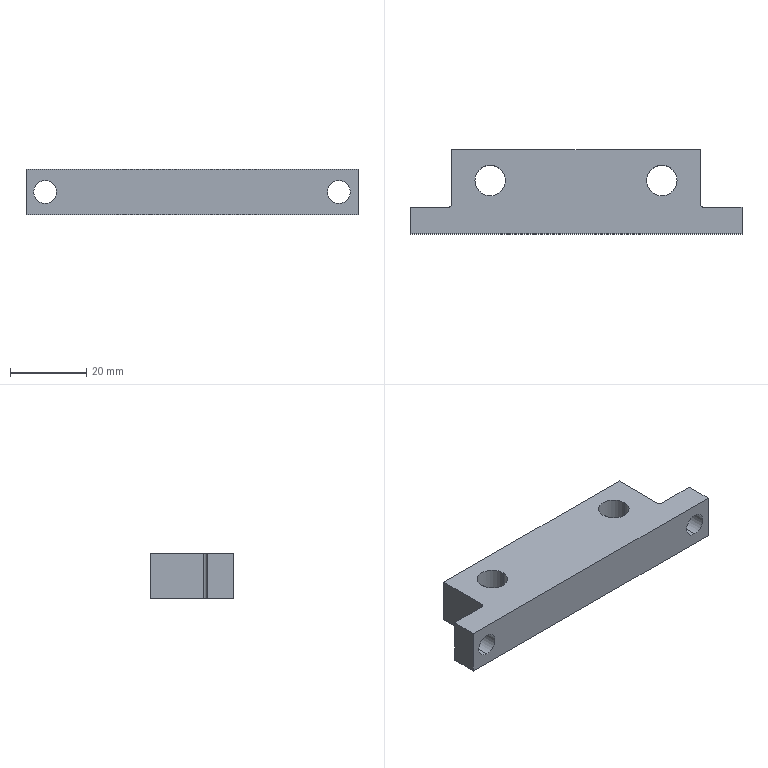Part | SolidWorks | features 3DProfileFeature 1, Extrusion 1, Fillet 1, HoleWzd 1, ICE 1, MirrorPattern 1 | 1 solid | 24 faces | box 87 x 22 x 12 mm | volume 17341 mm3 | cylinder 14 | plane 10 | commonest cylinder face diameters 3.3 x4 6 x4 8 x4 2 x2
STEP:
#1=CARTESIAN_POINT('',(-38.5,-22.,3.));
#2=VERTEX_POINT('',#1);
#3=CARTESIAN_POINT('',(-38.5,-22.,-3.));
#4=VERTEX_POINT('',#3);
#5=CARTESIAN_POINT('',(-38.5,-22.,0.));
#6=DIRECTION('',(0.,-1.,0.));
#7=DIRECTION('',(0.,0.,1.));
#8=AXIS2_PLACEMENT_3D('',#5,#6,#7);
#9=CIRCLE('',#8,3.);
#10=EDGE_CURVE('',#2,#4,#9,.T.);
#11=ORIENTED_EDGE('',*,*,#10,.T.);
#12=CARTESIAN_POINT('',(-38.5,-15.,-3.));
#13=VERTEX_POINT('',#12);
#14=CARTESIAN_POINT('',(-38.5,-22.001,-3.));
#15=DIRECTION('',(0.,1.,0.));
#16=VECTOR('',#15,1000.);
#17=LINE('',#14,#16);
#18=EDGE_CURVE('',#4,#13,#17,.T.);
#19=ORIENTED_EDGE('',*,*,#18,.T.);
#20=CARTESIAN_POINT('',(-38.5,-15.,3.));
#21=VERTEX_POINT('',#20);
#22=CARTESIAN_POINT('',(-38.5,-15.,0.));
#23=DIRECTION('',(0.,1.,0.));
#24=DIRECTION('',(0.,0.,1.));
#25=AXIS2_PLACEMENT_3D('',#22,#23,#24);
#26=CIRCLE('',#25,3.);
#27=EDGE_CURVE('',#13,#21,#26,.T.);
#28=ORIENTED_EDGE('',*,*,#27,.T.);
#29=CARTESIAN_POINT('',(-38.5,-22.001,3.));
#30=DIRECTION('',(0.,1.,0.));
#31=VECTOR('',#30,1000.);
#32=LINE('',#29,#31);
#33=EDGE_CURVE('',#2,#21,#32,.T.);
#34=ORIENTED_EDGE('',*,*,#33,.F.);
#35=EDGE_LOOP('',(#11,#19,#28,#34));
#36=FACE_OUTER_BOUND('',#35,.T.);
#37=CARTESIAN_POINT('',(-38.5,-22.001,0.));
#38=DIRECTION('',(0.,1.,0.));
#39=DIRECTION('',(0.,0.,1.));
#40=AXIS2_PLACEMENT_3D('',#37,#38,#39);
#41=CYLINDRICAL_SURFACE('',#40,3.);
#42=ADVANCED_FACE('',(#36),#41,.F.);
#43=CARTESIAN_POINT('',(38.5,-22.,3.));
#44=VERTEX_POINT('',#43);
#45=CARTESIAN_POINT('',(38.5,-22.,-3.));
#46=VERTEX_POINT('',#45);
#47=CARTESIAN_POINT('',(38.5,-22.,0.));
#48=DIRECTION('',(0.,-1.,0.));
#49=DIRECTION('',(0.,0.,1.));
#50=AXIS2_PLACEMENT_3D('',#47,#48,#49);
#51=CIRCLE('',#50,3.);
#52=EDGE_CURVE('',#44,#46,#51,.T.);
#53=ORIENTED_EDGE('',*,*,#52,.T.);
#54=CARTESIAN_POINT('',(38.5,-15.,-3.));
#55=VERTEX_POINT('',#54);
#56=CARTESIAN_POINT('',(38.5,-22.001,-3.));
#57=DIRECTION('',(0.,1.,0.));
#58=VECTOR('',#57,1000.);
#59=LINE('',#56,#58);
#60=EDGE_CURVE('',#46,#55,#59,.T.);
#61=ORIENTED_EDGE('',*,*,#60,.T.);
#62=CARTESIAN_POINT('',(38.5,-15.,3.));
#63=VERTEX_POINT('',#62);
#64=CARTESIAN_POINT('',(38.5,-15.,0.));
#65=DIRECTION('',(0.,1.,0.));
#66=DIRECTION('',(0.,0.,1.));
#67=AXIS2_PLACEMENT_3D('',#64,#65,#66);
#68=CIRCLE('',#67,3.);
#69=EDGE_CURVE('',#55,#63,#68,.T.);
#70=ORIENTED_EDGE('',*,*,#69,.T.);
#71=CARTESIAN_POINT('',(38.5,-22.001,3.));
#72=DIRECTION('',(0.,1.,0.));
#73=VECTOR('',#72,1000.);
#74=LINE('',#71,#73);
#75=EDGE_CURVE('',#44,#63,#74,.T.);
#76=ORIENTED_EDGE('',*,*,#75,.F.);
#77=EDGE_LOOP('',(#53,#61,#70,#76));
#78=FACE_OUTER_BOUND('',#77,.T.);
#79=CARTESIAN_POINT('',(38.5,-22.001,0.));
#80=DIRECTION('',(0.,1.,0.));
#81=DIRECTION('',(0.,0.,1.));
#82=AXIS2_PLACEMENT_3D('',#79,#80,#81);
#83=CYLINDRICAL_SURFACE('',#82,3.);
#84=ADVANCED_FACE('',(#78),#83,.F.);
#85=CARTESIAN_POINT('',(22.5,-4.,1.65));
#86=VERTEX_POINT('',#85);
#87=CARTESIAN_POINT('',(22.5,-4.,-1.65));
#88=VERTEX_POINT('',#87);
#89=CARTESIAN_POINT('',(22.5,-4.,1.65));
#90=CARTESIAN_POINT('',(22.39,-4.,1.65));
#91=CARTESIAN_POINT('',(22.281,-4.005,1.639));
#92=CARTESIAN_POINT('',(22.069,-4.022,1.596));
#93=CARTESIAN_POINT('',(21.963,-4.035,1.564));
#94=CARTESIAN_POINT('',(21.664,-4.083,1.439));
#95=CARTESIAN_POINT('',(21.483,-4.128,1.316));
#96=CARTESIAN_POINT('',(21.182,-4.22,1.015));
#97=CARTESIAN_POINT('',(21.06,-4.267,0.8337));
#98=CARTESIAN_POINT('',(20.936,-4.318,0.5367));
#99=CARTESIAN_POINT('',(20.904,-4.332,0.4315));
#100=CARTESIAN_POINT('',(20.861,-4.351,0.218));
#101=CARTESIAN_POINT('',(20.85,-4.356,0.1101));
#102=CARTESIAN_POINT('',(20.85,-4.356,-0.108));
#103=CARTESIAN_POINT('',(20.861,-4.351,-0.2186));
#104=CARTESIAN_POINT('',(20.904,-4.332,-0.4314));
#105=CARTESIAN_POINT('',(20.935,-4.318,-0.5352));
#106=CARTESIAN_POINT('',(21.019,-4.284,-0.736));
#107=CARTESIAN_POINT('',(21.07,-4.264,-0.8304));
#108=CARTESIAN_POINT('',(21.189,-4.22,-1.008));
#109=CARTESIAN_POINT('',(21.258,-4.197,-1.092));
#110=CARTESIAN_POINT('',(21.409,-4.151,-1.243));
#111=CARTESIAN_POINT('',(21.491,-4.128,-1.31));
#112=CARTESIAN_POINT('',(21.67,-4.086,-1.43));
#113=CARTESIAN_POINT('',(21.766,-4.067,-1.481));
#114=CARTESIAN_POINT('',(22.063,-4.019,-1.606));
#115=CARTESIAN_POINT('',(22.283,-4.,-1.65));
#116=CARTESIAN_POINT('',(22.5,-4.,-1.65));
#117=B_SPLINE_CURVE_WITH_KNOTS('',3,(#89,#90,#91,#92,#93,#94,#95,#96,#97,#98,#99,#100,#101,#102,#103,#104,#105,#106,#107,#108,#109,#110,#111,#112,#113,#114,#115,#116),.UNSPECIFIED.,.F.,.F.,(4,2,2,2,2,2,2,2,2,2,2,2,2,4),(0.,0.0003261,0.0006522,0.001304,0.001957,0.002283,0.002609,0.002935,0.003261,0.003587,0.003913,0.004239,0.004565,0.005218),.UNSPECIFIED.);
#118=EDGE_CURVE('',#86,#88,#117,.T.);
#119=ORIENTED_EDGE('',*,*,#118,.T.);
#120=CARTESIAN_POINT('',(22.5,0.,-1.65));
#121=VERTEX_POINT('',#120);
#122=CARTESIAN_POINT('',(22.5,0.,-1.65));
#123=DIRECTION('',(0.,1.,0.));
#124=VECTOR('',#123,1000.);
#125=LINE('',#122,#124);
#126=EDGE_CURVE('',#88,#121,#125,.T.);
#127=ORIENTED_EDGE('',*,*,#126,.T.);
#128=CARTESIAN_POINT('',(22.5,0.,1.65));
#129=VERTEX_POINT('',#128);
#130=CARTESIAN_POINT('',(22.5,0.,0.));
#131=DIRECTION('',(0.,1.,0.));
#132=DIRECTION('',(0.,0.,1.));
#133=AXIS2_PLACEMENT_3D('',#130,#131,#132);
#134=CIRCLE('',#133,1.65);
#135=EDGE_CURVE('',#121,#129,#134,.T.);
#136=ORIENTED_EDGE('',*,*,#135,.T.);
#137=CARTESIAN_POINT('',(22.5,0.,1.65));
#138=DIRECTION('',(0.,1.,0.));
#139=VECTOR('',#138,1000.);
#140=LINE('',#137,#139);
#141=EDGE_CURVE('',#86,#129,#140,.T.);
#142=ORIENTED_EDGE('',*,*,#141,.F.);
#143=EDGE_LOOP('',(#119,#127,#136,#142));
#144=FACE_OUTER_BOUND('',#143,.T.);
#145=CARTESIAN_POINT('',(22.5,0.,0.));
#146=DIRECTION('',(0.,1.,0.));
#147=DIRECTION('',(0.,0.,1.));
#148=AXIS2_PLACEMENT_3D('',#145,#146,#147);
#149=CYLINDRICAL_SURFACE('',#148,1.65);
#150=ADVANCED_FACE('',(#144),#149,.F.);
#151=CARTESIAN_POINT('',(-22.5,-4.,1.65));
#152=VERTEX_POINT('',#151);
#153=CARTESIAN_POINT('',(-22.5,-4.,-1.65));
#154=VERTEX_POINT('',#153);
#155=CARTESIAN_POINT('',(-22.5,-4.,1.65));
#156=CARTESIAN_POINT('',(-22.61,-4.,1.65));
#157=CARTESIAN_POINT('',(-22.719,-4.005,1.639));
#158=CARTESIAN_POINT('',(-22.931,-4.022,1.596));
#159=CARTESIAN_POINT('',(-23.037,-4.035,1.564));
#160=CARTESIAN_POINT('',(-23.336,-4.083,1.439));
#161=CARTESIAN_POINT('',(-23.517,-4.128,1.316));
#162=CARTESIAN_POINT('',(-23.818,-4.22,1.015));
#163=CARTESIAN_POINT('',(-23.94,-4.267,0.8337));
#164=CARTESIAN_POINT('',(-24.064,-4.318,0.5367));
#165=CARTESIAN_POINT('',(-24.096,-4.332,0.4315));
#166=CARTESIAN_POINT('',(-24.139,-4.351,0.218));
#167=CARTESIAN_POINT('',(-24.15,-4.356,0.1101));
#168=CARTESIAN_POINT('',(-24.15,-4.356,-0.108));
#169=CARTESIAN_POINT('',(-24.139,-4.351,-0.2186));
#170=CARTESIAN_POINT('',(-24.096,-4.332,-0.4314));
#171=CARTESIAN_POINT('',(-24.065,-4.318,-0.5352));
#172=CARTESIAN_POINT('',(-23.981,-4.284,-0.736));
#173=CARTESIAN_POINT('',(-23.93,-4.264,-0.8304));
#174=CARTESIAN_POINT('',(-23.811,-4.22,-1.008));
#175=CARTESIAN_POINT('',(-23.742,-4.197,-1.092));
#176=CARTESIAN_POINT('',(-23.591,-4.151,-1.243));
#177=CARTESIAN_POINT('',(-23.509,-4.128,-1.31));
#178=CARTESIAN_POINT('',(-23.33,-4.086,-1.43));
#179=CARTESIAN_POINT('',(-23.234,-4.067,-1.481));
#180=CARTESIAN_POINT('',(-22.937,-4.019,-1.606));
#181=CARTESIAN_POINT('',(-22.717,-4.,-1.65));
#182=CARTESIAN_POINT('',(-22.5,-4.,-1.65));
#183=B_SPLINE_CURVE_WITH_KNOTS('',3,(#155,#156,#157,#158,#159,#160,#161,#162,#163,#164,#165,#166,#167,#168,#169,#170,#171,#172,#173,#174,#175,#176,#177,#178,#179,#180,#181,#182),.UNSPECIFIED.,.F.,.F.,(4,2,2,2,2,2,2,2,2,2,2,2,2,4),(0.,0.0003261,0.0006522,0.001304,0.001957,0.002283,0.002609,0.002935,0.003261,0.003587,0.003913,0.004239,0.004565,0.005218),.UNSPECIFIED.);
#184=EDGE_CURVE('',#152,#154,#183,.T.);
#185=ORIENTED_EDGE('',*,*,#184,.T.);
#186=CARTESIAN_POINT('',(-22.5,0.,-1.65));
#187=VERTEX_POINT('',#186);
#188=CARTESIAN_POINT('',(-22.5,0.,-1.65));
#189=DIRECTION('',(0.,1.,0.));
#190=VECTOR('',#189,1000.);
#191=LINE('',#188,#190);
#192=EDGE_CURVE('',#154,#187,#191,.T.);
#193=ORIENTED_EDGE('',*,*,#192,.T.);
#194=CARTESIAN_POINT('',(-22.5,0.,1.65));
#195=VERTEX_POINT('',#194);
#196=CARTESIAN_POINT('',(-22.5,0.,0.));
#197=DIRECTION('',(0.,1.,0.));
#198=DIRECTION('',(0.,0.,1.));
#199=AXIS2_PLACEMENT_3D('',#196,#197,#198);
#200=CIRCLE('',#199,1.65);
#201=EDGE_CURVE('',#187,#195,#200,.T.);
#202=ORIENTED_EDGE('',*,*,#201,.T.);
#203=CARTESIAN_POINT('',(-22.5,0.,1.65));
#204=DIRECTION('',(0.,1.,0.));
#205=VECTOR('',#204,1000.);
#206=LINE('',#203,#205);
#207=EDGE_CURVE('',#152,#195,#206,.T.);
#208=ORIENTED_EDGE('',*,*,#207,.F.);
#209=EDGE_LOOP('',(#185,#193,#202,#208));
#210=FACE_OUTER_BOUND('',#209,.T.);
#211=CARTESIAN_POINT('',(-22.5,0.,0.));
#212=DIRECTION('',(0.,1.,0.));
#213=DIRECTION('',(0.,0.,1.));
#214=AXIS2_PLACEMENT_3D('',#211,#212,#213);
#215=CYLINDRICAL_SURFACE('',#214,1.65);
#216=ADVANCED_FACE('',(#210),#215,.F.);
#217=CARTESIAN_POINT('',(18.5,-8.,6.));
#218=VERTEX_POINT('',#217);
#219=CARTESIAN_POINT('',(26.5,-8.,6.));
#220=VERTEX_POINT('',#219);
#221=CARTESIAN_POINT('',(22.5,-8.,6.));
#222=DIRECTION('',(0.,0.,1.));
#223=DIRECTION('',(1.,0.,0.));
#224=AXIS2_PLACEMENT_3D('',#221,#222,#223);
#225=CIRCLE('',#224,4.);
#226=EDGE_CURVE('',#218,#220,#225,.T.);
#227=ORIENTED_EDGE('',*,*,#226,.T.);
#228=CARTESIAN_POINT('',(26.5,-8.,-6.));
#229=VERTEX_POINT('',#228);
#230=CARTESIAN_POINT('',(26.5,-8.,6.));
#231=DIRECTION('',(0.,0.,-1.));
#232=VECTOR('',#231,1000.);
#233=LINE('',#230,#232);
#234=EDGE_CURVE('',#220,#229,#233,.T.);
#235=ORIENTED_EDGE('',*,*,#234,.T.);
#236=CARTESIAN_POINT('',(18.5,-8.,-6.));
#237=VERTEX_POINT('',#236);
#238=CARTESIAN_POINT('',(22.5,-8.,-6.));
#239=DIRECTION('',(0.,0.,1.));
#240=DIRECTION('',(1.,0.,0.));
#241=AXIS2_PLACEMENT_3D('',#238,#239,#240);
#242=CIRCLE('',#241,4.);
#243=EDGE_CURVE('',#237,#229,#242,.T.);
#244=ORIENTED_EDGE('',*,*,#243,.F.);
#245=CARTESIAN_POINT('',(18.5,-8.,6.));
#246=DIRECTION('',(0.,0.,-1.));
#247=VECTOR('',#246,1000.);
#248=LINE('',#245,#247);
#249=EDGE_CURVE('',#218,#237,#248,.T.);
#250=ORIENTED_EDGE('',*,*,#249,.F.);
#251=EDGE_LOOP('',(#227,#235,#244,#250));
#252=FACE_OUTER_BOUND('',#251,.T.);
#253=CARTESIAN_POINT('',(22.5,-8.,6.));
#254=DIRECTION('',(0.,0.,-1.));
#255=DIRECTION('',(-1.,0.,0.));
#256=AXIS2_PLACEMENT_3D('',#253,#254,#255);
#257=CYLINDRICAL_SURFACE('',#256,4.);
#258=ADVANCED_FACE('',(#252),#257,.F.);
#259=CARTESIAN_POINT('',(-26.5,-8.,6.));
#260=VERTEX_POINT('',#259);
#261=CARTESIAN_POINT('',(-18.5,-8.,6.));
#262=VERTEX_POINT('',#261);
#263=CARTESIAN_POINT('',(-22.5,-8.,6.));
#264=DIRECTION('',(0.,0.,1.));
#265=DIRECTION('',(1.,0.,0.));
#266=AXIS2_PLACEMENT_3D('',#263,#264,#265);
#267=CIRCLE('',#266,4.);
#268=EDGE_CURVE('',#260,#262,#267,.T.);
#269=ORIENTED_EDGE('',*,*,#268,.T.);
#270=CARTESIAN_POINT('',(-18.5,-8.,-6.));
#271=VERTEX_POINT('',#270);
#272=CARTESIAN_POINT('',(-18.5,-8.,6.));
#273=DIRECTION('',(0.,0.,-1.));
#274=VECTOR('',#273,1000.);
#275=LINE('',#272,#274);
#276=EDGE_CURVE('',#262,#271,#275,.T.);
#277=ORIENTED_EDGE('',*,*,#276,.T.);
#278=CARTESIAN_POINT('',(-26.5,-8.,-6.));
#279=VERTEX_POINT('',#278);
#280=CARTESIAN_POINT('',(-22.5,-8.,-6.));
#281=DIRECTION('',(0.,0.,1.));
#282=DIRECTION('',(1.,0.,0.));
#283=AXIS2_PLACEMENT_3D('',#280,#281,#282);
#284=CIRCLE('',#283,4.);
#285=EDGE_CURVE('',#279,#271,#284,.T.);
#286=ORIENTED_EDGE('',*,*,#285,.F.);
#287=CARTESIAN_POINT('',(-26.5,-8.,6.));
#288=DIRECTION('',(0.,0.,-1.));
#289=VECTOR('',#288,1000.);
#290=LINE('',#287,#289);
#291=EDGE_CURVE('',#260,#279,#290,.T.);
#292=ORIENTED_EDGE('',*,*,#291,.F.);
#293=EDGE_LOOP('',(#269,#277,#286,#292));
#294=FACE_OUTER_BOUND('',#293,.T.);
#295=CARTESIAN_POINT('',(-22.5,-8.,6.));
#296=DIRECTION('',(0.,0.,-1.));
#297=DIRECTION('',(-1.,0.,0.));
#298=AXIS2_PLACEMENT_3D('',#295,#296,#297);
#299=CYLINDRICAL_SURFACE('',#298,4.);
#300=ADVANCED_FACE('',(#294),#299,.F.);
#301=ORIENTED_EDGE('',*,*,#268,.F.);
#302=CARTESIAN_POINT('',(-22.5,-8.,6.));
#303=DIRECTION('',(0.,0.,1.));
#304=DIRECTION('',(1.,0.,0.));
#305=AXIS2_PLACEMENT_3D('',#302,#303,#304);
#306=CIRCLE('',#305,4.);
#307=EDGE_CURVE('',#262,#260,#306,.T.);
#308=ORIENTED_EDGE('',*,*,#307,.F.);
#309=EDGE_LOOP('',(#301,#308));
#310=FACE_BOUND('',#309,.T.);
#311=CARTESIAN_POINT('',(32.5,0.,6.));
#312=VERTEX_POINT('',#311);
#313=CARTESIAN_POINT('',(-32.5,0.,6.));
#314=VERTEX_POINT('',#313);
#315=CARTESIAN_POINT('',(32.5,0.,6.));
#316=DIRECTION('',(-1.,0.,0.));
#317=VECTOR('',#316,1000.);
#318=LINE('',#315,#317);
#319=EDGE_CURVE('',#312,#314,#318,.T.);
#320=ORIENTED_EDGE('',*,*,#319,.T.);
#321=CARTESIAN_POINT('',(-32.5,-14.,6.));
#322=VERTEX_POINT('',#321);
#323=CARTESIAN_POINT('',(-32.5,0.,6.));
#324=DIRECTION('',(0.,-1.,0.));
#325=VECTOR('',#324,1000.);
#326=LINE('',#323,#325);
#327=EDGE_CURVE('',#314,#322,#326,.T.);
#328=ORIENTED_EDGE('',*,*,#327,.T.);
#329=CARTESIAN_POINT('',(-33.5,-15.,6.));
#330=VERTEX_POINT('',#329);
#331=CARTESIAN_POINT('',(-33.5,-14.,6.));
#332=DIRECTION('',(0.,0.,-1.));
#333=DIRECTION('',(1.,0.,0.));
#334=AXIS2_PLACEMENT_3D('',#331,#332,#333);
#335=CIRCLE('',#334,1.);
#336=EDGE_CURVE('',#322,#330,#335,.T.);
#337=ORIENTED_EDGE('',*,*,#336,.T.);
#338=CARTESIAN_POINT('',(-43.5,-15.,6.));
#339=VERTEX_POINT('',#338);
#340=CARTESIAN_POINT('',(-32.5,-15.,6.));
#341=DIRECTION('',(-1.,0.,0.));
#342=VECTOR('',#341,1000.);
#343=LINE('',#340,#342);
#344=EDGE_CURVE('',#330,#339,#343,.T.);
#345=ORIENTED_EDGE('',*,*,#344,.T.);
#346=CARTESIAN_POINT('',(-43.5,-22.,6.));
#347=VERTEX_POINT('',#346);
#348=CARTESIAN_POINT('',(-43.5,-15.,6.));
#349=DIRECTION('',(0.,-1.,0.));
#350=VECTOR('',#349,1000.);
#351=LINE('',#348,#350);
#352=EDGE_CURVE('',#339,#347,#351,.T.);
#353=ORIENTED_EDGE('',*,*,#352,.T.);
#354=CARTESIAN_POINT('',(43.5,-22.,6.));
#355=VERTEX_POINT('',#354);
#356=CARTESIAN_POINT('',(-43.5,-22.,6.));
#357=DIRECTION('',(1.,0.,0.));
#358=VECTOR('',#357,1000.);
#359=LINE('',#356,#358);
#360=EDGE_CURVE('',#347,#355,#359,.T.);
#361=ORIENTED_EDGE('',*,*,#360,.T.);
#362=CARTESIAN_POINT('',(43.5,-15.,6.));
#363=VERTEX_POINT('',#362);
#364=CARTESIAN_POINT('',(43.5,-22.,6.));
#365=DIRECTION('',(0.,1.,0.));
#366=VECTOR('',#365,1000.);
#367=LINE('',#364,#366);
#368=EDGE_CURVE('',#355,#363,#367,.T.);
#369=ORIENTED_EDGE('',*,*,#368,.T.);
#370=CARTESIAN_POINT('',(33.5,-15.,6.));
#371=VERTEX_POINT('',#370);
#372=CARTESIAN_POINT('',(43.5,-15.,6.));
#373=DIRECTION('',(-1.,0.,0.));
#374=VECTOR('',#373,1000.);
#375=LINE('',#372,#374);
#376=EDGE_CURVE('',#363,#371,#375,.T.);
#377=ORIENTED_EDGE('',*,*,#376,.T.);
#378=CARTESIAN_POINT('',(32.5,-14.,6.));
#379=VERTEX_POINT('',#378);
#380=CARTESIAN_POINT('',(33.5,-14.,6.));
#381=DIRECTION('',(0.,0.,-1.));
#382=DIRECTION('',(1.,0.,0.));
#383=AXIS2_PLACEMENT_3D('',#380,#381,#382);
#384=CIRCLE('',#383,1.);
#385=EDGE_CURVE('',#371,#379,#384,.T.);
#386=ORIENTED_EDGE('',*,*,#385,.T.);
#387=CARTESIAN_POINT('',(32.5,-15.,6.));
#388=DIRECTION('',(0.,1.,0.));
#389=VECTOR('',#388,1000.);
#390=LINE('',#387,#389);
#391=EDGE_CURVE('',#379,#312,#390,.T.);
#392=ORIENTED_EDGE('',*,*,#391,.T.);
#393=EDGE_LOOP('',(#320,#328,#337,#345,#353,#361,#369,#377,#386,#392));
#394=FACE_OUTER_BOUND('',#393,.T.);
#395=ORIENTED_EDGE('',*,*,#226,.F.);
#396=CARTESIAN_POINT('',(22.5,-8.,6.));
#397=DIRECTION('',(0.,0.,1.));
#398=DIRECTION('',(1.,0.,0.));
#399=AXIS2_PLACEMENT_3D('',#396,#397,#398);
#400=CIRCLE('',#399,4.);
#401=EDGE_CURVE('',#220,#218,#400,.T.);
#402=ORIENTED_EDGE('',*,*,#401,.F.);
#403=EDGE_LOOP('',(#395,#402));
#404=FACE_BOUND('',#403,.T.);
#405=CARTESIAN_POINT('',(0.,0.,6.));
#406=DIRECTION('',(0.,0.,1.));
#407=DIRECTION('',(1.,0.,0.));
#408=AXIS2_PLACEMENT_3D('',#405,#406,#407);
#409=PLANE('',#408);
#410=ADVANCED_FACE('',(#310,#394,#404),#409,.T.);
#411=CARTESIAN_POINT('',(32.5,0.,-6.));
#412=VERTEX_POINT('',#411);
#413=CARTESIAN_POINT('',(-32.5,0.,-6.));
#414=VERTEX_POINT('',#413);
#415=CARTESIAN_POINT('',(0.,0.,-6.));
#416=DIRECTION('',(-1.,0.,0.));
#417=VECTOR('',#416,1000.);
#418=LINE('',#415,#417);
#419=EDGE_CURVE('',#412,#414,#418,.T.);
#420=ORIENTED_EDGE('',*,*,#419,.F.);
#421=CARTESIAN_POINT('',(32.5,-14.,-6.));
#422=VERTEX_POINT('',#421);
#423=CARTESIAN_POINT('',(32.5,-15.,-6.));
#424=DIRECTION('',(0.,1.,0.));
#425=VECTOR('',#424,1000.);
#426=LINE('',#423,#425);
#427=EDGE_CURVE('',#422,#412,#426,.T.);
#428=ORIENTED_EDGE('',*,*,#427,.F.);
#429=CARTESIAN_POINT('',(33.5,-15.,-6.));
#430=VERTEX_POINT('',#429);
#431=CARTESIAN_POINT('',(33.5,-14.,-6.));
#432=DIRECTION('',(0.,0.,1.));
#433=DIRECTION('',(1.,0.,0.));
#434=AXIS2_PLACEMENT_3D('',#431,#432,#433);
#435=CIRCLE('',#434,1.);
#436=EDGE_CURVE('',#422,#430,#435,.T.);
#437=ORIENTED_EDGE('',*,*,#436,.T.);
#438=CARTESIAN_POINT('',(43.5,-15.,-6.));
#439=VERTEX_POINT('',#438);
#440=CARTESIAN_POINT('',(43.5,-15.,-6.));
#441=DIRECTION('',(-1.,0.,0.));
#442=VECTOR('',#441,1000.);
#443=LINE('',#440,#442);
#444=EDGE_CURVE('',#439,#430,#443,.T.);
#445=ORIENTED_EDGE('',*,*,#444,.F.);
#446=CARTESIAN_POINT('',(43.5,-22.,-6.));
#447=VERTEX_POINT('',#446);
#448=CARTESIAN_POINT('',(43.5,-22.,-6.));
#449=DIRECTION('',(0.,1.,0.));
#450=VECTOR('',#449,1000.);
#451=LINE('',#448,#450);
#452=EDGE_CURVE('',#447,#439,#451,.T.);
#453=ORIENTED_EDGE('',*,*,#452,.F.);
#454=CARTESIAN_POINT('',(-43.5,-22.,-6.));
#455=VERTEX_POINT('',#454);
#456=CARTESIAN_POINT('',(-43.5,-22.,-6.));
#457=DIRECTION('',(1.,0.,0.));
#458=VECTOR('',#457,1000.);
#459=LINE('',#456,#458);
#460=EDGE_CURVE('',#455,#447,#459,.T.);
#461=ORIENTED_EDGE('',*,*,#460,.F.);
#462=CARTESIAN_POINT('',(-43.5,-15.,-6.));
#463=VERTEX_POINT('',#462);
#464=CARTESIAN_POINT('',(-43.5,-15.,-6.));
#465=DIRECTION('',(0.,-1.,0.));
#466=VECTOR('',#465,1000.);
#467=LINE('',#464,#466);
#468=EDGE_CURVE('',#463,#455,#467,.T.);
#469=ORIENTED_EDGE('',*,*,#468,.F.);
#470=CARTESIAN_POINT('',(-33.5,-15.,-6.));
#471=VERTEX_POINT('',#470);
#472=CARTESIAN_POINT('',(-32.5,-15.,-6.));
#473=DIRECTION('',(-1.,0.,0.));
#474=VECTOR('',#473,1000.);
#475=LINE('',#472,#474);
#476=EDGE_CURVE('',#471,#463,#475,.T.);
#477=ORIENTED_EDGE('',*,*,#476,.F.);
#478=CARTESIAN_POINT('',(-32.5,-14.,-6.));
#479=VERTEX_POINT('',#478);
#480=CARTESIAN_POINT('',(-33.5,-14.,-6.));
#481=DIRECTION('',(0.,0.,1.));
#482=DIRECTION('',(1.,0.,0.));
#483=AXIS2_PLACEMENT_3D('',#480,#481,#482);
#484=CIRCLE('',#483,1.);
#485=EDGE_CURVE('',#471,#479,#484,.T.);
#486=ORIENTED_EDGE('',*,*,#485,.T.);
#487=CARTESIAN_POINT('',(-32.5,0.,-6.));
#488=DIRECTION('',(0.,-1.,0.));
#489=VECTOR('',#488,1000.);
#490=LINE('',#487,#489);
#491=EDGE_CURVE('',#414,#479,#490,.T.);
#492=ORIENTED_EDGE('',*,*,#491,.F.);
#493=EDGE_LOOP('',(#420,#428,#437,#445,#453,#461,#469,#477,#486,#492));
#494=FACE_OUTER_BOUND('',#493,.T.);
#495=ORIENTED_EDGE('',*,*,#285,.T.);
#496=CARTESIAN_POINT('',(-22.5,-8.,-6.));
#497=DIRECTION('',(0.,0.,1.));
#498=DIRECTION('',(1.,0.,0.));
#499=AXIS2_PLACEMENT_3D('',#496,#497,#498);
#500=CIRCLE('',#499,4.);
#501=EDGE_CURVE('',#271,#279,#500,.T.);
#502=ORIENTED_EDGE('',*,*,#501,.T.);
#503=EDGE_LOOP('',(#495,#502));
#504=FACE_BOUND('',#503,.T.);
#505=ORIENTED_EDGE('',*,*,#243,.T.);
#506=CARTESIAN_POINT('',(22.5,-8.,-6.));
#507=DIRECTION('',(0.,0.,1.));
#508=DIRECTION('',(1.,0.,0.));
#509=AXIS2_PLACEMENT_3D('',#506,#507,#508);
#510=CIRCLE('',#509,4.);
#511=EDGE_CURVE('',#229,#237,#510,.T.);
#512=ORIENTED_EDGE('',*,*,#511,.T.);
#513=EDGE_LOOP('',(#505,#512));
#514=FACE_BOUND('',#513,.T.);
#515=CARTESIAN_POINT('',(0.,0.,-6.));
#516=DIRECTION('',(0.,0.,1.));
#517=DIRECTION('',(1.,0.,0.));
#518=AXIS2_PLACEMENT_3D('',#515,#516,#517);
#519=PLANE('',#518);
#520=ADVANCED_FACE('',(#494,#504,#514),#519,.F.);
#521=CARTESIAN_POINT('',(22.5,0.,0.));
#522=DIRECTION('',(0.,1.,0.));
#523=DIRECTION('',(0.,0.,1.));
#524=AXIS2_PLACEMENT_3D('',#521,#522,#523);
#525=CIRCLE('',#524,1.65);
#526=EDGE_CURVE('',#129,#121,#525,.T.);
#527=ORIENTED_EDGE('',*,*,#526,.F.);
#528=ORIENTED_EDGE('',*,*,#135,.F.);
#529=EDGE_LOOP('',(#527,#528));
#530=FACE_BOUND('',#529,.T.);
#531=CARTESIAN_POINT('',(-22.5,0.,0.));
#532=DIRECTION('',(0.,1.,0.));
#533=DIRECTION('',(0.,0.,1.));
#534=AXIS2_PLACEMENT_3D('',#531,#532,#533);
#535=CIRCLE('',#534,1.65);
#536=EDGE_CURVE('',#195,#187,#535,.T.);
#537=ORIENTED_EDGE('',*,*,#536,.F.);
#538=ORIENTED_EDGE('',*,*,#201,.F.);
#539=EDGE_LOOP('',(#537,#538));
#540=FACE_BOUND('',#539,.T.);
#541=ORIENTED_EDGE('',*,*,#419,.T.);
#542=CARTESIAN_POINT('',(-32.5,0.,6.));
#543=DIRECTION('',(0.,0.,-1.));
#544=VECTOR('',#543,1000.);
#545=LINE('',#542,#544);
#546=EDGE_CURVE('',#314,#414,#545,.T.);
#547=ORIENTED_EDGE('',*,*,#546,.F.);
#548=ORIENTED_EDGE('',*,*,#319,.F.);
#549=CARTESIAN_POINT('',(32.5,0.,6.));
#550=DIRECTION('',(0.,0.,-1.));
#551=VECTOR('',#550,1000.);
#552=LINE('',#549,#551);
#553=EDGE_CURVE('',#312,#412,#552,.T.);
#554=ORIENTED_EDGE('',*,*,#553,.T.);
#555=EDGE_LOOP('',(#541,#547,#548,#554));
#556=FACE_OUTER_BOUND('',#555,.T.);
#557=CARTESIAN_POINT('',(0.,0.,6.));
#558=DIRECTION('',(0.,-1.,0.));
#559=DIRECTION('',(1.,0.,0.));
#560=AXIS2_PLACEMENT_3D('',#557,#558,#559);
#561=PLANE('',#560);
#562=ADVANCED_FACE('',(#530,#540,#556),#561,.F.);
#563=ORIENTED_EDGE('',*,*,#491,.T.);
#564=CARTESIAN_POINT('',(-32.5,-14.,6.));
#565=DIRECTION('',(0.,0.,1.));
#566=VECTOR('',#565,1000.);
#567=LINE('',#564,#566);
#568=EDGE_CURVE('',#479,#322,#567,.T.);
#569=ORIENTED_EDGE('',*,*,#568,.T.);
#570=ORIENTED_EDGE('',*,*,#327,.F.);
#571=ORIENTED_EDGE('',*,*,#546,.T.);
#572=EDGE_LOOP('',(#563,#569,#570,#571));
#573=FACE_OUTER_BOUND('',#572,.T.);
#574=CARTESIAN_POINT('',(-32.5,0.,6.));
#575=DIRECTION('',(1.,0.,0.));
#576=DIRECTION('',(0.,0.,-1.));
#577=AXIS2_PLACEMENT_3D('',#574,#575,#576);
#578=PLANE('',#577);
#579=ADVANCED_FACE('',(#573),#578,.F.);
#580=CARTESIAN_POINT('',(-38.5,-15.,0.));
#581=DIRECTION('',(0.,1.,0.));
#582=DIRECTION('',(0.,0.,1.));
#583=AXIS2_PLACEMENT_3D('',#580,#581,#582);
#584=CIRCLE('',#583,3.);
#585=EDGE_CURVE('',#21,#13,#584,.T.);
#586=ORIENTED_EDGE('',*,*,#585,.F.);
#587=ORIENTED_EDGE('',*,*,#27,.F.);
#588=EDGE_LOOP('',(#586,#587));
#589=FACE_BOUND('',#588,.T.);
#590=ORIENTED_EDGE('',*,*,#344,.F.);
#591=CARTESIAN_POINT('',(-33.5,-15.,-6.));
#592=DIRECTION('',(0.,0.,-1.));
#593=VECTOR('',#592,1000.);
#594=LINE('',#591,#593);
#595=EDGE_CURVE('',#330,#471,#594,.T.);
#596=ORIENTED_EDGE('',*,*,#595,.T.);
#597=ORIENTED_EDGE('',*,*,#476,.T.);
#598=CARTESIAN_POINT('',(-43.5,-15.,6.));
#599=DIRECTION('',(0.,0.,-1.));
#600=VECTOR('',#599,1000.);
#601=LINE('',#598,#600);
#602=EDGE_CURVE('',#339,#463,#601,.T.);
#603=ORIENTED_EDGE('',*,*,#602,.F.);
#604=EDGE_LOOP('',(#590,#596,#597,#603));
#605=FACE_OUTER_BOUND('',#604,.T.);
#606=CARTESIAN_POINT('',(-32.5,-15.,6.));
#607=DIRECTION('',(0.,-1.,0.));
#608=DIRECTION('',(0.,0.,-1.));
#609=AXIS2_PLACEMENT_3D('',#606,#607,#608);
#610=PLANE('',#609);
#611=ADVANCED_FACE('',(#589,#605),#610,.F.);
#612=ORIENTED_EDGE('',*,*,#468,.T.);
#613=CARTESIAN_POINT('',(-43.5,-22.,6.));
#614=DIRECTION('',(0.,0.,-1.));
#615=VECTOR('',#614,1000.);
#616=LINE('',#613,#615);
#617=EDGE_CURVE('',#347,#455,#616,.T.);
#618=ORIENTED_EDGE('',*,*,#617,.F.);
#619=ORIENTED_EDGE('',*,*,#352,.F.);
#620=ORIENTED_EDGE('',*,*,#602,.T.);
#621=EDGE_LOOP('',(#612,#618,#619,#620));
#622=FACE_OUTER_BOUND('',#621,.T.);
#623=CARTESIAN_POINT('',(-43.5,-15.,6.));
#624=DIRECTION('',(1.,0.,0.));
#625=DIRECTION('',(0.,0.,-1.));
#626=AXIS2_PLACEMENT_3D('',#623,#624,#625);
#627=PLANE('',#626);
#628=ADVANCED_FACE('',(#622),#627,.F.);
#629=ORIENTED_EDGE('',*,*,#10,.F.);
#630=CARTESIAN_POINT('',(-38.5,-22.,0.));
#631=DIRECTION('',(0.,-1.,0.));
#632=DIRECTION('',(0.,0.,1.));
#633=AXIS2_PLACEMENT_3D('',#630,#631,#632);
#634=CIRCLE('',#633,3.);
#635=EDGE_CURVE('',#4,#2,#634,.T.);
#636=ORIENTED_EDGE('',*,*,#635,.F.);
#637=EDGE_LOOP('',(#629,#636));
#638=FACE_BOUND('',#637,.T.);
#639=ORIENTED_EDGE('',*,*,#52,.F.);
#640=CARTESIAN_POINT('',(38.5,-22.,0.));
#641=DIRECTION('',(0.,-1.,0.));
#642=DIRECTION('',(0.,0.,1.));
#643=AXIS2_PLACEMENT_3D('',#640,#641,#642);
#644=CIRCLE('',#643,3.);
#645=EDGE_CURVE('',#46,#44,#644,.T.);
#646=ORIENTED_EDGE('',*,*,#645,.F.);
#647=EDGE_LOOP('',(#639,#646));
#648=FACE_BOUND('',#647,.T.);
#649=ORIENTED_EDGE('',*,*,#460,.T.);
#650=CARTESIAN_POINT('',(43.5,-22.,6.));
#651=DIRECTION('',(0.,0.,-1.));
#652=VECTOR('',#651,1000.);
#653=LINE('',#650,#652);
#654=EDGE_CURVE('',#355,#447,#653,.T.);
#655=ORIENTED_EDGE('',*,*,#654,.F.);
#656=ORIENTED_EDGE('',*,*,#360,.F.);
#657=ORIENTED_EDGE('',*,*,#617,.T.);
#658=EDGE_LOOP('',(#649,#655,#656,#657));
#659=FACE_OUTER_BOUND('',#658,.T.);
#660=CARTESIAN_POINT('',(-43.5,-22.,6.));
#661=DIRECTION('',(0.,1.,0.));
#662=DIRECTION('',(0.,0.,1.));
#663=AXIS2_PLACEMENT_3D('',#660,#661,#662);
#664=PLANE('',#663);
#665=ADVANCED_FACE('',(#638,#648,#659),#664,.F.);
#666=ORIENTED_EDGE('',*,*,#452,.T.);
#667=CARTESIAN_POINT('',(43.5,-15.,6.));
#668=DIRECTION('',(0.,0.,-1.));
#669=VECTOR('',#668,1000.);
#670=LINE('',#667,#669);
#671=EDGE_CURVE('',#363,#439,#670,.T.);
#672=ORIENTED_EDGE('',*,*,#671,.F.);
#673=ORIENTED_EDGE('',*,*,#368,.F.);
#674=ORIENTED_EDGE('',*,*,#654,.T.);
#675=EDGE_LOOP('',(#666,#672,#673,#674));
#676=FACE_OUTER_BOUND('',#675,.T.);
#677=CARTESIAN_POINT('',(43.5,-22.,6.));
#678=DIRECTION('',(-1.,0.,0.));
#679=DIRECTION('',(0.,0.,1.));
#680=AXIS2_PLACEMENT_3D('',#677,#678,#679);
#681=PLANE('',#680);
#682=ADVANCED_FACE('',(#676),#681,.F.);
#683=CARTESIAN_POINT('',(38.5,-15.,0.));
#684=DIRECTION('',(0.,1.,0.));
#685=DIRECTION('',(0.,0.,1.));
#686=AXIS2_PLACEMENT_3D('',#683,#684,#685);
#687=CIRCLE('',#686,3.);
#688=EDGE_CURVE('',#63,#55,#687,.T.);
#689=ORIENTED_EDGE('',*,*,#688,.F.);
#690=ORIENTED_EDGE('',*,*,#69,.F.);
#691=EDGE_LOOP('',(#689,#690));
#692=FACE_BOUND('',#691,.T.);
#693=ORIENTED_EDGE('',*,*,#444,.T.);
#694=CARTESIAN_POINT('',(33.5,-15.,6.));
#695=DIRECTION('',(0.,0.,1.));
#696=VECTOR('',#695,1000.);
#697=LINE('',#694,#696);
#698=EDGE_CURVE('',#430,#371,#697,.T.);
#699=ORIENTED_EDGE('',*,*,#698,.T.);
#700=ORIENTED_EDGE('',*,*,#376,.F.);
#701=ORIENTED_EDGE('',*,*,#671,.T.);
#702=EDGE_LOOP('',(#693,#699,#700,#701));
#703=FACE_OUTER_BOUND('',#702,.T.);
#704=CARTESIAN_POINT('',(43.5,-15.,6.));
#705=DIRECTION('',(0.,-1.,0.));
#706=DIRECTION('',(1.,0.,0.));
#707=AXIS2_PLACEMENT_3D('',#704,#705,#706);
#708=PLANE('',#707);
#709=ADVANCED_FACE('',(#692,#703),#708,.F.);
#710=ORIENTED_EDGE('',*,*,#391,.F.);
#711=CARTESIAN_POINT('',(32.5,-14.,-6.));
#712=DIRECTION('',(0.,0.,-1.));
#713=VECTOR('',#712,1000.);
#714=LINE('',#711,#713);
#715=EDGE_CURVE('',#379,#422,#714,.T.);
#716=ORIENTED_EDGE('',*,*,#715,.T.);
#717=ORIENTED_EDGE('',*,*,#427,.T.);
#718=ORIENTED_EDGE('',*,*,#553,.F.);
#719=EDGE_LOOP('',(#710,#716,#717,#718));
#720=FACE_OUTER_BOUND('',#719,.T.);
#721=CARTESIAN_POINT('',(32.5,-15.,6.));
#722=DIRECTION('',(-1.,0.,0.));
#723=DIRECTION('',(0.,0.,1.));
#724=AXIS2_PLACEMENT_3D('',#721,#722,#723);
#725=PLANE('',#724);
#726=ADVANCED_FACE('',(#720),#725,.F.);
#727=ORIENTED_EDGE('',*,*,#276,.F.);
#728=ORIENTED_EDGE('',*,*,#307,.T.);
#729=ORIENTED_EDGE('',*,*,#291,.T.);
#730=ORIENTED_EDGE('',*,*,#501,.F.);
#731=EDGE_LOOP('',(#727,#728,#729,#730));
#732=FACE_OUTER_BOUND('',#731,.T.);
#733=ORIENTED_EDGE('',*,*,#184,.F.);
#734=CARTESIAN_POINT('',(-22.5,-4.,-1.65));
#735=CARTESIAN_POINT('',(-22.391,-4.,-1.65));
#736=CARTESIAN_POINT('',(-22.281,-4.005,-1.639));
#737=CARTESIAN_POINT('',(-22.067,-4.022,-1.596));
#738=CARTESIAN_POINT('',(-21.964,-4.035,-1.564));
#739=CARTESIAN_POINT('',(-21.665,-4.083,-1.439));
#740=CARTESIAN_POINT('',(-21.484,-4.128,-1.318));
#741=CARTESIAN_POINT('',(-21.256,-4.197,-1.09));
#742=CARTESIAN_POINT('',(-21.189,-4.22,-1.008));
#743=CARTESIAN_POINT('',(-21.07,-4.264,-0.8304));
#744=CARTESIAN_POINT('',(-21.019,-4.284,-0.7344));
#745=CARTESIAN_POINT('',(-20.936,-4.318,-0.5355));
#746=CARTESIAN_POINT('',(-20.904,-4.332,-0.4326));
#747=CARTESIAN_POINT('',(-20.861,-4.351,-0.2198));
#748=CARTESIAN_POINT('',(-20.85,-4.356,-0.1091));
#749=CARTESIAN_POINT('',(-20.85,-4.356,0.2172));
#750=CARTESIAN_POINT('',(-20.894,-4.335,0.4362));
#751=CARTESIAN_POINT('',(-21.018,-4.284,0.7343));
#752=CARTESIAN_POINT('',(-21.07,-4.264,0.8304));
#753=CARTESIAN_POINT('',(-21.189,-4.22,1.008));
#754=CARTESIAN_POINT('',(-21.257,-4.197,1.09));
#755=CARTESIAN_POINT('',(-21.408,-4.151,1.242));
#756=CARTESIAN_POINT('',(-21.492,-4.128,1.311));
#757=CARTESIAN_POINT('',(-21.669,-4.086,1.429));
#758=CARTESIAN_POINT('',(-21.763,-4.067,1.48));
#759=CARTESIAN_POINT('',(-22.065,-4.018,1.607));
#760=CARTESIAN_POINT('',(-22.279,-4.,1.65));
#761=CARTESIAN_POINT('',(-22.5,-4.,1.65));
#762=B_SPLINE_CURVE_WITH_KNOTS('',3,(#734,#735,#736,#737,#738,#739,#740,#741,#742,#743,#744,#745,#746,#747,#748,#749,#750,#751,#752,#753,#754,#755,#756,#757,#758,#759,#760,#761),.UNSPECIFIED.,.F.,.F.,(4,2,2,2,2,2,2,2,2,2,2,2,2,4),(0.005218,0.005543,0.005869,0.006521,0.006847,0.007173,0.007499,0.007824,0.008476,0.008802,0.009128,0.009454,0.009779,0.01043),.UNSPECIFIED.);
#763=EDGE_CURVE('',#154,#152,#762,.T.);
#764=ORIENTED_EDGE('',*,*,#763,.F.);
#765=EDGE_LOOP('',(#733,#764));
#766=FACE_BOUND('',#765,.T.);
#767=CARTESIAN_POINT('',(-22.5,-8.,6.));
#768=DIRECTION('',(0.,0.,-1.));
#769=DIRECTION('',(-1.,0.,0.));
#770=AXIS2_PLACEMENT_3D('',#767,#768,#769);
#771=CYLINDRICAL_SURFACE('',#770,4.);
#772=ADVANCED_FACE('',(#732,#766),#771,.F.);
#773=ORIENTED_EDGE('',*,*,#234,.F.);
#774=ORIENTED_EDGE('',*,*,#401,.T.);
#775=ORIENTED_EDGE('',*,*,#249,.T.);
#776=ORIENTED_EDGE('',*,*,#511,.F.);
#777=EDGE_LOOP('',(#773,#774,#775,#776));
#778=FACE_OUTER_BOUND('',#777,.T.);
#779=ORIENTED_EDGE('',*,*,#118,.F.);
#780=CARTESIAN_POINT('',(22.5,-4.,-1.65));
#781=CARTESIAN_POINT('',(22.609,-4.,-1.65));
#782=CARTESIAN_POINT('',(22.719,-4.005,-1.639));
#783=CARTESIAN_POINT('',(22.933,-4.022,-1.596));
#784=CARTESIAN_POINT('',(23.036,-4.035,-1.564));
#785=CARTESIAN_POINT('',(23.335,-4.083,-1.439));
#786=CARTESIAN_POINT('',(23.516,-4.128,-1.318));
#787=CARTESIAN_POINT('',(23.744,-4.197,-1.09));
#788=CARTESIAN_POINT('',(23.811,-4.22,-1.008));
#789=CARTESIAN_POINT('',(23.93,-4.264,-0.8304));
#790=CARTESIAN_POINT('',(23.981,-4.284,-0.7344));
#791=CARTESIAN_POINT('',(24.064,-4.318,-0.5355));
#792=CARTESIAN_POINT('',(24.096,-4.332,-0.4326));
#793=CARTESIAN_POINT('',(24.139,-4.351,-0.2198));
#794=CARTESIAN_POINT('',(24.15,-4.356,-0.1091));
#795=CARTESIAN_POINT('',(24.15,-4.356,0.2172));
#796=CARTESIAN_POINT('',(24.106,-4.335,0.4362));
#797=CARTESIAN_POINT('',(23.982,-4.284,0.7343));
#798=CARTESIAN_POINT('',(23.93,-4.264,0.8304));
#799=CARTESIAN_POINT('',(23.811,-4.22,1.008));
#800=CARTESIAN_POINT('',(23.743,-4.197,1.09));
#801=CARTESIAN_POINT('',(23.592,-4.151,1.242));
#802=CARTESIAN_POINT('',(23.508,-4.128,1.311));
#803=CARTESIAN_POINT('',(23.331,-4.086,1.429));
#804=CARTESIAN_POINT('',(23.237,-4.067,1.48));
#805=CARTESIAN_POINT('',(22.935,-4.018,1.607));
#806=CARTESIAN_POINT('',(22.721,-4.,1.65));
#807=CARTESIAN_POINT('',(22.5,-4.,1.65));
#808=B_SPLINE_CURVE_WITH_KNOTS('',3,(#780,#781,#782,#783,#784,#785,#786,#787,#788,#789,#790,#791,#792,#793,#794,#795,#796,#797,#798,#799,#800,#801,#802,#803,#804,#805,#806,#807),.UNSPECIFIED.,.F.,.F.,(4,2,2,2,2,2,2,2,2,2,2,2,2,4),(0.005218,0.005543,0.005869,0.006521,0.006847,0.007173,0.007499,0.007824,0.008476,0.008802,0.009128,0.009454,0.009779,0.01043),.UNSPECIFIED.);
#809=EDGE_CURVE('',#88,#86,#808,.T.);
#810=ORIENTED_EDGE('',*,*,#809,.F.);
#811=EDGE_LOOP('',(#779,#810));
#812=FACE_BOUND('',#811,.T.);
#813=CARTESIAN_POINT('',(22.5,-8.,6.));
#814=DIRECTION('',(0.,0.,-1.));
#815=DIRECTION('',(-1.,0.,0.));
#816=AXIS2_PLACEMENT_3D('',#813,#814,#815);
#817=CYLINDRICAL_SURFACE('',#816,4.);
#818=ADVANCED_FACE('',(#778,#812),#817,.F.);
#819=ORIENTED_EDGE('',*,*,#192,.F.);
#820=ORIENTED_EDGE('',*,*,#763,.T.);
#821=ORIENTED_EDGE('',*,*,#207,.T.);
#822=ORIENTED_EDGE('',*,*,#536,.T.);
#823=EDGE_LOOP('',(#819,#820,#821,#822));
#824=FACE_OUTER_BOUND('',#823,.T.);
#825=CARTESIAN_POINT('',(-22.5,0.,0.));
#826=DIRECTION('',(0.,1.,0.));
#827=DIRECTION('',(0.,0.,1.));
#828=AXIS2_PLACEMENT_3D('',#825,#826,#827);
#829=CYLINDRICAL_SURFACE('',#828,1.65);
#830=ADVANCED_FACE('',(#824),#829,.F.);
#831=ORIENTED_EDGE('',*,*,#126,.F.);
#832=ORIENTED_EDGE('',*,*,#809,.T.);
#833=ORIENTED_EDGE('',*,*,#141,.T.);
#834=ORIENTED_EDGE('',*,*,#526,.T.);
#835=EDGE_LOOP('',(#831,#832,#833,#834));
#836=FACE_OUTER_BOUND('',#835,.T.);
#837=CARTESIAN_POINT('',(22.5,0.,0.));
#838=DIRECTION('',(0.,1.,0.));
#839=DIRECTION('',(0.,0.,1.));
#840=AXIS2_PLACEMENT_3D('',#837,#838,#839);
#841=CYLINDRICAL_SURFACE('',#840,1.65);
#842=ADVANCED_FACE('',(#836),#841,.F.);
#843=ORIENTED_EDGE('',*,*,#385,.F.);
#844=ORIENTED_EDGE('',*,*,#698,.F.);
#845=ORIENTED_EDGE('',*,*,#436,.F.);
#846=ORIENTED_EDGE('',*,*,#715,.F.);
#847=EDGE_LOOP('',(#843,#844,#845,#846));
#848=FACE_OUTER_BOUND('',#847,.T.);
#849=CARTESIAN_POINT('',(33.5,-14.,6.));
#850=DIRECTION('',(0.,0.,1.));
#851=DIRECTION('',(1.,0.,0.));
#852=AXIS2_PLACEMENT_3D('',#849,#850,#851);
#853=CYLINDRICAL_SURFACE('',#852,1.);
#854=ADVANCED_FACE('',(#848),#853,.F.);
#855=ORIENTED_EDGE('',*,*,#336,.F.);
#856=ORIENTED_EDGE('',*,*,#568,.F.);
#857=ORIENTED_EDGE('',*,*,#485,.F.);
#858=ORIENTED_EDGE('',*,*,#595,.F.);
#859=EDGE_LOOP('',(#855,#856,#857,#858));
#860=FACE_OUTER_BOUND('',#859,.T.);
#861=CARTESIAN_POINT('',(-33.5,-14.,6.));
#862=DIRECTION('',(0.,0.,1.));
#863=DIRECTION('',(1.,0.,0.));
#864=AXIS2_PLACEMENT_3D('',#861,#862,#863);
#865=CYLINDRICAL_SURFACE('',#864,1.);
#866=ADVANCED_FACE('',(#860),#865,.F.);
#867=ORIENTED_EDGE('',*,*,#60,.F.);
#868=ORIENTED_EDGE('',*,*,#645,.T.);
#869=ORIENTED_EDGE('',*,*,#75,.T.);
#870=ORIENTED_EDGE('',*,*,#688,.T.);
#871=EDGE_LOOP('',(#867,#868,#869,#870));
#872=FACE_OUTER_BOUND('',#871,.T.);
#873=CARTESIAN_POINT('',(38.5,-22.001,0.));
#874=DIRECTION('',(0.,1.,0.));
#875=DIRECTION('',(0.,0.,1.));
#876=AXIS2_PLACEMENT_3D('',#873,#874,#875);
#877=CYLINDRICAL_SURFACE('',#876,3.);
#878=ADVANCED_FACE('',(#872),#877,.F.);
#879=ORIENTED_EDGE('',*,*,#18,.F.);
#880=ORIENTED_EDGE('',*,*,#635,.T.);
#881=ORIENTED_EDGE('',*,*,#33,.T.);
#882=ORIENTED_EDGE('',*,*,#585,.T.);
#883=EDGE_LOOP('',(#879,#880,#881,#882));
#884=FACE_OUTER_BOUND('',#883,.T.);
#885=CARTESIAN_POINT('',(-38.5,-22.001,0.));
#886=DIRECTION('',(0.,1.,0.));
#887=DIRECTION('',(0.,0.,1.));
#888=AXIS2_PLACEMENT_3D('',#885,#886,#887);
#889=CYLINDRICAL_SURFACE('',#888,3.);
#890=ADVANCED_FACE('',(#884),#889,.F.);
#891=CLOSED_SHELL('',(#42,#84,#150,#216,#258,#300,#410,#520,#562,#579,#611,#628,#665,#682,#709,#726,#772,#818,#830,#842,#854,#866,#878,#890));
#892=MANIFOLD_SOLID_BREP('',#891);
#893=CARTESIAN_POINT('',(0.,0.,0.));
#894=DIRECTION('',(0.,0.,1.));
#895=DIRECTION('',(1.,0.,0.));
#896=AXIS2_PLACEMENT_3D('',#893,#894,#895);
#897=(LENGTH_UNIT()NAMED_UNIT(*)SI_UNIT(.MILLI.,.METRE.));
#898=UNCERTAINTY_MEASURE_WITH_UNIT(LENGTH_MEASURE(0.00001),#897,'','');
#899=(NAMED_UNIT(*)PLANE_ANGLE_UNIT()SI_UNIT($,.RADIAN.));
#900=(NAMED_UNIT(*)SI_UNIT($,.STERADIAN.)SOLID_ANGLE_UNIT());
#901=(GEOMETRIC_REPRESENTATION_CONTEXT(3)GLOBAL_UNCERTAINTY_ASSIGNED_CONTEXT((#898))GLOBAL_UNIT_ASSIGNED_CONTEXT((#897,#899,#900))REPRESENTATION_CONTEXT('',''));
#902=ADVANCED_BREP_SHAPE_REPRESENTATION('',(#892,#896),#901);